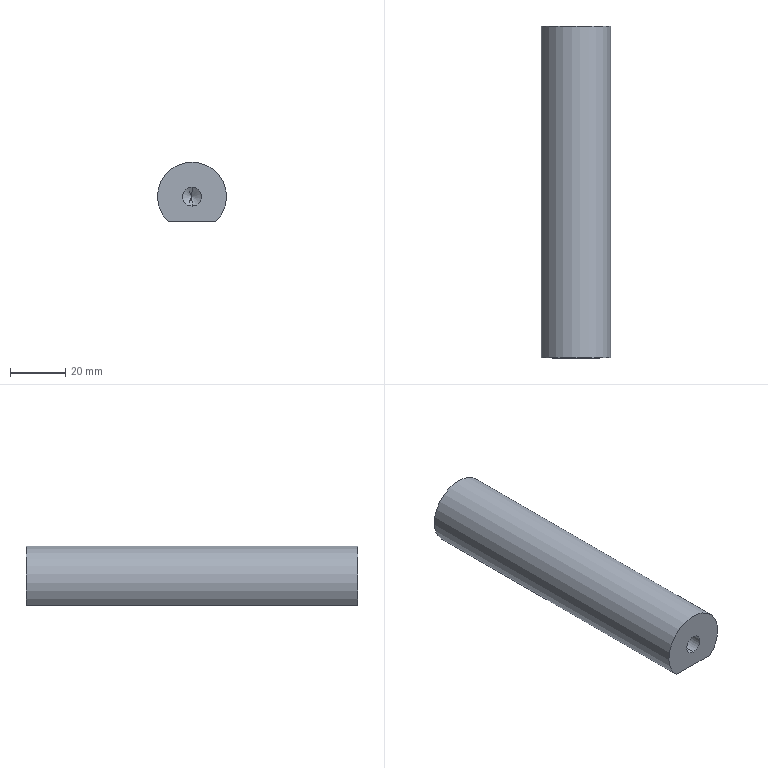Part | STEP file | PN_0003 | 1 solid | 12 faces | box 25 x 120 x 21.5 mm | volume 52408 mm3 | cylinder 5 | cone 4 | plane 3 | commonest cylinder face diameters 6.8 x4 25 x1
STEP:
#1=CARTESIAN_POINT('',(0.,0.,0.));
#2=DIRECTION('',(0.,0.,1.));
#3=DIRECTION('',(1.,0.,0.));
#4=AXIS2_PLACEMENT_3D('',#1,#2,#3);
#5=CARTESIAN_POINT('',(0.,19.75,-3.4));
#6=VERTEX_POINT('',#5);
#7=CARTESIAN_POINT('',(0.,0.,-3.4));
#8=VERTEX_POINT('',#7);
#9=CARTESIAN_POINT('',(0.,0.,-3.4));
#10=DIRECTION('',(0.,-1.,0.));
#11=VECTOR('',#10,1.);
#12=LINE('',#9,#11);
#13=CARTESIAN_POINT('',(0.,0.,0.));
#14=DIRECTION('',(0.,-1.,0.));
#15=DIRECTION('',(0.,0.,-1.));
#16=AXIS2_PLACEMENT_3D('',#13,#14,#15);
#17=CYLINDRICAL_SURFACE('',#16,3.4);
#18=CARTESIAN_POINT('',(6.283,0.));
#19=DIRECTION('',(0.,1.));
#20=VECTOR('',#19,1.);
#21=LINE('',#18,#20);
#22=(GEOMETRIC_REPRESENTATION_CONTEXT(2)PARAMETRIC_REPRESENTATION_CONTEXT()REPRESENTATION_CONTEXT('',''));
#23=DEFINITIONAL_REPRESENTATION('',(#21),#22);
#24=PCURVE('',#17,#23);
#25=CARTESIAN_POINT('',(0.,0.,0.));
#26=DIRECTION('',(0.,-1.,0.));
#27=DIRECTION('',(0.,0.,-1.));
#28=AXIS2_PLACEMENT_3D('',#25,#26,#27);
#29=CYLINDRICAL_SURFACE('',#28,3.4);
#30=CARTESIAN_POINT('',(0.,0.));
#31=DIRECTION('',(0.,1.));
#32=VECTOR('',#31,1.);
#33=LINE('',#30,#32);
#34=(GEOMETRIC_REPRESENTATION_CONTEXT(2)PARAMETRIC_REPRESENTATION_CONTEXT()REPRESENTATION_CONTEXT('',''));
#35=DEFINITIONAL_REPRESENTATION('',(#33),#34);
#36=PCURVE('',#29,#35);
#37=SURFACE_CURVE('',#12,(#24,#36),.PCURVE_S1.);
#38=EDGE_CURVE('',#6,#8,#37,.T.);
#39=ORIENTED_EDGE('',*,*,#38,.T.);
#40=CARTESIAN_POINT('',(0.,0.,3.4));
#41=VERTEX_POINT('',#40);
#42=CARTESIAN_POINT('',(0.,0.,0.));
#43=DIRECTION('',(0.,-1.,0.));
#44=DIRECTION('',(0.,0.,-1.));
#45=AXIS2_PLACEMENT_3D('',#42,#43,#44);
#46=CIRCLE('',#45,3.4);
#47=CARTESIAN_POINT('',(0.,0.));
#48=DIRECTION('',(1.,0.));
#49=VECTOR('',#48,1.);
#50=LINE('',#47,#49);
#51=(GEOMETRIC_REPRESENTATION_CONTEXT(2)PARAMETRIC_REPRESENTATION_CONTEXT()REPRESENTATION_CONTEXT('',''));
#52=DEFINITIONAL_REPRESENTATION('',(#50),#51);
#53=PCURVE('',#17,#52);
#54=CARTESIAN_POINT('',(0.,0.,0.));
#55=DIRECTION('',(0.,1.,0.));
#56=DIRECTION('',(0.,0.,1.));
#57=AXIS2_PLACEMENT_3D('',#54,#55,#56);
#58=PLANE('',#57);
#59=CARTESIAN_POINT('',(-3.4,0.));
#60=CARTESIAN_POINT('',(-3.4,5.889));
#61=CARTESIAN_POINT('',(1.7,2.944));
#62=CARTESIAN_POINT('',(6.8,0.));
#63=CARTESIAN_POINT('',(1.7,-2.944));
#64=CARTESIAN_POINT('',(-3.4,-5.889));
#65=CARTESIAN_POINT('',(-3.4,0.));
#66=(BOUNDED_CURVE()B_SPLINE_CURVE(2,(#59,#60,#61,#62,#63,#64,#65),.UNSPECIFIED.,.T.,.F.)B_SPLINE_CURVE_WITH_KNOTS((1,2,2,2,2,1),(-2.094,0.,2.094,4.189,6.283,8.378),.UNSPECIFIED.)CURVE()GEOMETRIC_REPRESENTATION_ITEM()RATIONAL_B_SPLINE_CURVE((1.,0.5,1.,0.5,1.,0.5,1.))REPRESENTATION_ITEM(''));
#67=(GEOMETRIC_REPRESENTATION_CONTEXT(2)PARAMETRIC_REPRESENTATION_CONTEXT()REPRESENTATION_CONTEXT('',''));
#68=DEFINITIONAL_REPRESENTATION('',(#66),#67);
#69=PCURVE('',#58,#68);
#70=SURFACE_CURVE('',#46,(#53,#69),.PCURVE_S1.);
#71=EDGE_CURVE('',#41,#8,#70,.T.);
#72=ORIENTED_EDGE('',*,*,#71,.F.);
#73=CARTESIAN_POINT('',(0.,19.75,3.4));
#74=VERTEX_POINT('',#73);
#75=CARTESIAN_POINT('',(0.,0.,3.4));
#76=DIRECTION('',(0.,-1.,0.));
#77=VECTOR('',#76,1.);
#78=LINE('',#75,#77);
#79=CARTESIAN_POINT('',(3.142,0.));
#80=DIRECTION('',(0.,1.));
#81=VECTOR('',#80,1.);
#82=LINE('',#79,#81);
#83=(GEOMETRIC_REPRESENTATION_CONTEXT(2)PARAMETRIC_REPRESENTATION_CONTEXT()REPRESENTATION_CONTEXT('',''));
#84=DEFINITIONAL_REPRESENTATION('',(#82),#83);
#85=PCURVE('',#17,#84);
#86=CARTESIAN_POINT('',(3.142,0.));
#87=DIRECTION('',(0.,1.));
#88=VECTOR('',#87,1.);
#89=LINE('',#86,#88);
#90=(GEOMETRIC_REPRESENTATION_CONTEXT(2)PARAMETRIC_REPRESENTATION_CONTEXT()REPRESENTATION_CONTEXT('',''));
#91=DEFINITIONAL_REPRESENTATION('',(#89),#90);
#92=PCURVE('',#29,#91);
#93=SURFACE_CURVE('',#78,(#85,#92),.PCURVE_S1.);
#94=EDGE_CURVE('',#74,#41,#93,.T.);
#95=ORIENTED_EDGE('',*,*,#94,.F.);
#96=CARTESIAN_POINT('',(0.,19.75,0.));
#97=DIRECTION('',(0.,-1.,0.));
#98=DIRECTION('',(0.,0.,-1.));
#99=AXIS2_PLACEMENT_3D('',#96,#97,#98);
#100=CIRCLE('',#99,3.4);
#101=CARTESIAN_POINT('',(0.,-19.75));
#102=DIRECTION('',(1.,0.));
#103=VECTOR('',#102,1.);
#104=LINE('',#101,#103);
#105=(GEOMETRIC_REPRESENTATION_CONTEXT(2)PARAMETRIC_REPRESENTATION_CONTEXT()REPRESENTATION_CONTEXT('',''));
#106=DEFINITIONAL_REPRESENTATION('',(#104),#105);
#107=PCURVE('',#17,#106);
#108=CARTESIAN_POINT('',(0.,19.75,0.));
#109=DIRECTION('',(0.,-1.,0.));
#110=DIRECTION('',(0.,0.,-1.));
#111=AXIS2_PLACEMENT_3D('',#108,#109,#110);
#112=CONICAL_SURFACE('',#111,3.4,1.03);
#113=CARTESIAN_POINT('',(0.,0.));
#114=DIRECTION('',(1.,0.));
#115=VECTOR('',#114,1.);
#116=LINE('',#113,#115);
#117=(GEOMETRIC_REPRESENTATION_CONTEXT(2)PARAMETRIC_REPRESENTATION_CONTEXT()REPRESENTATION_CONTEXT('',''));
#118=DEFINITIONAL_REPRESENTATION('',(#116),#117);
#119=PCURVE('',#112,#118);
#120=SURFACE_CURVE('',#100,(#107,#119),.PCURVE_S1.);
#121=EDGE_CURVE('',#74,#6,#120,.T.);
#122=ORIENTED_EDGE('',*,*,#121,.T.);
#123=EDGE_LOOP('',(#39,#72,#95,#122));
#124=FACE_BOUND('',#123,.F.);
#125=ADVANCED_FACE('',(#124),#17,.F.);
#126=ORIENTED_EDGE('',*,*,#121,.F.);
#127=CARTESIAN_POINT('',(0.,21.793,0.));
#128=VERTEX_POINT('',#127);
#129=CARTESIAN_POINT('',(0.,19.75,3.4));
#130=DIRECTION('',(0.,-0.515,0.8572));
#131=VECTOR('',#130,1.);
#132=LINE('',#129,#131);
#133=CARTESIAN_POINT('',(3.142,0.));
#134=DIRECTION('',(0.,1.));
#135=VECTOR('',#134,1.);
#136=LINE('',#133,#135);
#137=(GEOMETRIC_REPRESENTATION_CONTEXT(2)PARAMETRIC_REPRESENTATION_CONTEXT()REPRESENTATION_CONTEXT('',''));
#138=DEFINITIONAL_REPRESENTATION('',(#136),#137);
#139=PCURVE('',#112,#138);
#140=CARTESIAN_POINT('',(0.,19.75,0.));
#141=DIRECTION('',(0.,-1.,0.));
#142=DIRECTION('',(0.,0.,-1.));
#143=AXIS2_PLACEMENT_3D('',#140,#141,#142);
#144=CONICAL_SURFACE('',#143,3.4,1.03);
#145=CARTESIAN_POINT('',(3.142,0.));
#146=DIRECTION('',(0.,1.));
#147=VECTOR('',#146,1.);
#148=LINE('',#145,#147);
#149=(GEOMETRIC_REPRESENTATION_CONTEXT(2)PARAMETRIC_REPRESENTATION_CONTEXT()REPRESENTATION_CONTEXT('',''));
#150=DEFINITIONAL_REPRESENTATION('',(#148),#149);
#151=PCURVE('',#144,#150);
#152=SURFACE_CURVE('',#132,(#139,#151),.PCURVE_S1.);
#153=EDGE_CURVE('',#128,#74,#152,.T.);
#154=ORIENTED_EDGE('',*,*,#153,.F.);
#155=CARTESIAN_POINT('',(0.,19.75,-3.4));
#156=DIRECTION('',(0.,-0.515,-0.8572));
#157=VECTOR('',#156,1.);
#158=LINE('',#155,#157);
#159=CARTESIAN_POINT('',(6.283,0.));
#160=DIRECTION('',(0.,1.));
#161=VECTOR('',#160,1.);
#162=LINE('',#159,#161);
#163=(GEOMETRIC_REPRESENTATION_CONTEXT(2)PARAMETRIC_REPRESENTATION_CONTEXT()REPRESENTATION_CONTEXT('',''));
#164=DEFINITIONAL_REPRESENTATION('',(#162),#163);
#165=PCURVE('',#112,#164);
#166=CARTESIAN_POINT('',(0.,0.));
#167=DIRECTION('',(0.,1.));
#168=VECTOR('',#167,1.);
#169=LINE('',#166,#168);
#170=(GEOMETRIC_REPRESENTATION_CONTEXT(2)PARAMETRIC_REPRESENTATION_CONTEXT()REPRESENTATION_CONTEXT('',''));
#171=DEFINITIONAL_REPRESENTATION('',(#169),#170);
#172=PCURVE('',#144,#171);
#173=SURFACE_CURVE('',#158,(#165,#172),.PCURVE_S1.);
#174=EDGE_CURVE('',#128,#6,#173,.T.);
#175=ORIENTED_EDGE('',*,*,#174,.T.);
#176=EDGE_LOOP('',(#126,#154,#175));
#177=FACE_BOUND('',#176,.F.);
#178=ADVANCED_FACE('',(#177),#112,.F.);
#179=CARTESIAN_POINT('',(0.,100.25,3.398));
#180=VERTEX_POINT('',#179);
#181=CARTESIAN_POINT('',(0.,120.,3.398));
#182=VERTEX_POINT('',#181);
#183=CARTESIAN_POINT('',(0.,120.,3.398));
#184=DIRECTION('',(0.,1.,0.));
#185=VECTOR('',#184,1.);
#186=LINE('',#183,#185);
#187=CARTESIAN_POINT('',(0.,120.,-0.002145));
#188=DIRECTION('',(0.,1.,0.));
#189=DIRECTION('',(0.,0.,1.));
#190=AXIS2_PLACEMENT_3D('',#187,#188,#189);
#191=CYLINDRICAL_SURFACE('',#190,3.4);
#192=CARTESIAN_POINT('',(6.283,0.));
#193=DIRECTION('',(0.,1.));
#194=VECTOR('',#193,1.);
#195=LINE('',#192,#194);
#196=(GEOMETRIC_REPRESENTATION_CONTEXT(2)PARAMETRIC_REPRESENTATION_CONTEXT()REPRESENTATION_CONTEXT('',''));
#197=DEFINITIONAL_REPRESENTATION('',(#195),#196);
#198=PCURVE('',#191,#197);
#199=CARTESIAN_POINT('',(0.,120.,-0.002145));
#200=DIRECTION('',(0.,1.,0.));
#201=DIRECTION('',(0.,0.,1.));
#202=AXIS2_PLACEMENT_3D('',#199,#200,#201);
#203=CYLINDRICAL_SURFACE('',#202,3.4);
#204=CARTESIAN_POINT('',(0.,0.));
#205=DIRECTION('',(0.,1.));
#206=VECTOR('',#205,1.);
#207=LINE('',#204,#206);
#208=(GEOMETRIC_REPRESENTATION_CONTEXT(2)PARAMETRIC_REPRESENTATION_CONTEXT()REPRESENTATION_CONTEXT('',''));
#209=DEFINITIONAL_REPRESENTATION('',(#207),#208);
#210=PCURVE('',#203,#209);
#211=SURFACE_CURVE('',#186,(#198,#210),.PCURVE_S1.);
#212=EDGE_CURVE('',#180,#182,#211,.T.);
#213=ORIENTED_EDGE('',*,*,#212,.T.);
#214=CARTESIAN_POINT('',(0.,120.,-3.402));
#215=VERTEX_POINT('',#214);
#216=CARTESIAN_POINT('',(0.,120.,-0.002145));
#217=DIRECTION('',(0.,1.,0.));
#218=DIRECTION('',(0.,0.,1.));
#219=AXIS2_PLACEMENT_3D('',#216,#217,#218);
#220=CIRCLE('',#219,3.4);
#221=CARTESIAN_POINT('',(0.,0.));
#222=DIRECTION('',(1.,0.));
#223=VECTOR('',#222,1.);
#224=LINE('',#221,#223);
#225=(GEOMETRIC_REPRESENTATION_CONTEXT(2)PARAMETRIC_REPRESENTATION_CONTEXT()REPRESENTATION_CONTEXT('',''));
#226=DEFINITIONAL_REPRESENTATION('',(#224),#225);
#227=PCURVE('',#191,#226);
#228=CARTESIAN_POINT('',(0.,120.,0.));
#229=DIRECTION('',(0.,1.,0.));
#230=DIRECTION('',(0.,0.,1.));
#231=AXIS2_PLACEMENT_3D('',#228,#229,#230);
#232=PLANE('',#231);
#233=CARTESIAN_POINT('',(-0.002145,0.));
#234=DIRECTION('',(1.,0.));
#235=AXIS2_PLACEMENT_2D('',#233,#234);
#236=CIRCLE('',#235,3.4);
#237=(GEOMETRIC_REPRESENTATION_CONTEXT(2)PARAMETRIC_REPRESENTATION_CONTEXT()REPRESENTATION_CONTEXT('',''));
#238=DEFINITIONAL_REPRESENTATION('',(#236),#237);
#239=PCURVE('',#232,#238);
#240=SURFACE_CURVE('',#220,(#227,#239),.PCURVE_S1.);
#241=EDGE_CURVE('',#215,#182,#240,.T.);
#242=ORIENTED_EDGE('',*,*,#241,.F.);
#243=CARTESIAN_POINT('',(0.,100.25,-3.402));
#244=VERTEX_POINT('',#243);
#245=CARTESIAN_POINT('',(0.,120.,-3.402));
#246=DIRECTION('',(0.,1.,0.));
#247=VECTOR('',#246,1.);
#248=LINE('',#245,#247);
#249=CARTESIAN_POINT('',(3.142,0.));
#250=DIRECTION('',(0.,1.));
#251=VECTOR('',#250,1.);
#252=LINE('',#249,#251);
#253=(GEOMETRIC_REPRESENTATION_CONTEXT(2)PARAMETRIC_REPRESENTATION_CONTEXT()REPRESENTATION_CONTEXT('',''));
#254=DEFINITIONAL_REPRESENTATION('',(#252),#253);
#255=PCURVE('',#191,#254);
#256=CARTESIAN_POINT('',(3.142,0.));
#257=DIRECTION('',(0.,1.));
#258=VECTOR('',#257,1.);
#259=LINE('',#256,#258);
#260=(GEOMETRIC_REPRESENTATION_CONTEXT(2)PARAMETRIC_REPRESENTATION_CONTEXT()REPRESENTATION_CONTEXT('',''));
#261=DEFINITIONAL_REPRESENTATION('',(#259),#260);
#262=PCURVE('',#203,#261);
#263=SURFACE_CURVE('',#248,(#255,#262),.PCURVE_S1.);
#264=EDGE_CURVE('',#244,#215,#263,.T.);
#265=ORIENTED_EDGE('',*,*,#264,.F.);
#266=CARTESIAN_POINT('',(0.,100.25,-0.002145));
#267=DIRECTION('',(0.,1.,0.));
#268=DIRECTION('',(0.,0.,1.));
#269=AXIS2_PLACEMENT_3D('',#266,#267,#268);
#270=CIRCLE('',#269,3.4);
#271=CARTESIAN_POINT('',(0.,-19.75));
#272=DIRECTION('',(1.,0.));
#273=VECTOR('',#272,1.);
#274=LINE('',#271,#273);
#275=(GEOMETRIC_REPRESENTATION_CONTEXT(2)PARAMETRIC_REPRESENTATION_CONTEXT()REPRESENTATION_CONTEXT('',''));
#276=DEFINITIONAL_REPRESENTATION('',(#274),#275);
#277=PCURVE('',#191,#276);
#278=CARTESIAN_POINT('',(0.,100.25,-0.002145));
#279=DIRECTION('',(0.,1.,0.));
#280=DIRECTION('',(0.,0.,1.));
#281=AXIS2_PLACEMENT_3D('',#278,#279,#280);
#282=CONICAL_SURFACE('',#281,3.4,1.03);
#283=CARTESIAN_POINT('',(0.,0.));
#284=DIRECTION('',(1.,0.));
#285=VECTOR('',#284,1.);
#286=LINE('',#283,#285);
#287=(GEOMETRIC_REPRESENTATION_CONTEXT(2)PARAMETRIC_REPRESENTATION_CONTEXT()REPRESENTATION_CONTEXT('',''));
#288=DEFINITIONAL_REPRESENTATION('',(#286),#287);
#289=PCURVE('',#282,#288);
#290=SURFACE_CURVE('',#270,(#277,#289),.PCURVE_S1.);
#291=EDGE_CURVE('',#244,#180,#290,.T.);
#292=ORIENTED_EDGE('',*,*,#291,.T.);
#293=EDGE_LOOP('',(#213,#242,#265,#292));
#294=FACE_BOUND('',#293,.F.);
#295=ADVANCED_FACE('',(#294),#191,.F.);
#296=ORIENTED_EDGE('',*,*,#291,.F.);
#297=CARTESIAN_POINT('',(0.,98.207,-0.002145));
#298=VERTEX_POINT('',#297);
#299=CARTESIAN_POINT('',(0.,100.25,-3.402));
#300=DIRECTION('',(0.,0.515,-0.8572));
#301=VECTOR('',#300,1.);
#302=LINE('',#299,#301);
#303=CARTESIAN_POINT('',(3.142,-2.043));
#304=CARTESIAN_POINT('',(3.142,-2.012));
#305=CARTESIAN_POINT('',(3.142,-1.95));
#306=CARTESIAN_POINT('',(3.142,-1.857));
#307=CARTESIAN_POINT('',(3.142,-1.764));
#308=CARTESIAN_POINT('',(3.142,-1.671));
#309=CARTESIAN_POINT('',(3.142,-1.579));
#310=CARTESIAN_POINT('',(3.142,-1.486));
#311=CARTESIAN_POINT('',(3.142,-1.393));
#312=CARTESIAN_POINT('',(3.142,-1.3));
#313=CARTESIAN_POINT('',(3.142,-1.207));
#314=CARTESIAN_POINT('',(3.142,-1.114));
#315=CARTESIAN_POINT('',(3.142,-1.021));
#316=CARTESIAN_POINT('',(3.142,-0.9286));
#317=CARTESIAN_POINT('',(3.142,-0.8357));
#318=CARTESIAN_POINT('',(3.142,-0.7429));
#319=CARTESIAN_POINT('',(3.142,-0.65));
#320=CARTESIAN_POINT('',(3.142,-0.5572));
#321=CARTESIAN_POINT('',(3.142,-0.4643));
#322=CARTESIAN_POINT('',(3.142,-0.3714));
#323=CARTESIAN_POINT('',(3.142,-0.2786));
#324=CARTESIAN_POINT('',(3.142,-0.1857));
#325=CARTESIAN_POINT('',(3.142,-0.09286));
#326=CARTESIAN_POINT('',(3.142,-0.03095));
#327=CARTESIAN_POINT('',(3.142,0.));
#328=B_SPLINE_CURVE_WITH_KNOTS('',3,(#303,#304,#305,#306,#307,#308,#309,#310,#311,#312,#313,#314,#315,#316,#317,#318,#319,#320,#321,#322,#323,#324,#325,#326,#327),.UNSPECIFIED.,.F.,.F.,(4,1,1,1,1,1,1,1,1,1,1,1,1,1,1,1,1,1,1,1,1,1,4),(-3.967,-3.786,-3.606,-3.426,-3.245,-3.065,-2.885,-2.704,-2.524,-2.344,-2.164,-1.983,-1.803,-1.623,-1.442,-1.262,-1.082,-0.9015,-0.7212,-0.5409,-0.3606,-0.1803,0.),.UNSPECIFIED.);
#329=(GEOMETRIC_REPRESENTATION_CONTEXT(2)PARAMETRIC_REPRESENTATION_CONTEXT()REPRESENTATION_CONTEXT('',''));
#330=DEFINITIONAL_REPRESENTATION('',(#328),#329);
#331=PCURVE('',#282,#330);
#332=CARTESIAN_POINT('',(0.,100.25,-0.002145));
#333=DIRECTION('',(0.,1.,0.));
#334=DIRECTION('',(0.,0.,1.));
#335=AXIS2_PLACEMENT_3D('',#332,#333,#334);
#336=CONICAL_SURFACE('',#335,3.4,1.03);
#337=CARTESIAN_POINT('',(3.142,-2.043));
#338=CARTESIAN_POINT('',(3.142,-2.012));
#339=CARTESIAN_POINT('',(3.142,-1.95));
#340=CARTESIAN_POINT('',(3.142,-1.857));
#341=CARTESIAN_POINT('',(3.142,-1.764));
#342=CARTESIAN_POINT('',(3.142,-1.671));
#343=CARTESIAN_POINT('',(3.142,-1.579));
#344=CARTESIAN_POINT('',(3.142,-1.486));
#345=CARTESIAN_POINT('',(3.142,-1.393));
#346=CARTESIAN_POINT('',(3.142,-1.3));
#347=CARTESIAN_POINT('',(3.142,-1.207));
#348=CARTESIAN_POINT('',(3.142,-1.114));
#349=CARTESIAN_POINT('',(3.142,-1.021));
#350=CARTESIAN_POINT('',(3.142,-0.9286));
#351=CARTESIAN_POINT('',(3.142,-0.8357));
#352=CARTESIAN_POINT('',(3.142,-0.7429));
#353=CARTESIAN_POINT('',(3.142,-0.65));
#354=CARTESIAN_POINT('',(3.142,-0.5572));
#355=CARTESIAN_POINT('',(3.142,-0.4643));
#356=CARTESIAN_POINT('',(3.142,-0.3714));
#357=CARTESIAN_POINT('',(3.142,-0.2786));
#358=CARTESIAN_POINT('',(3.142,-0.1857));
#359=CARTESIAN_POINT('',(3.142,-0.09286));
#360=CARTESIAN_POINT('',(3.142,-0.03095));
#361=CARTESIAN_POINT('',(3.142,0.));
#362=B_SPLINE_CURVE_WITH_KNOTS('',3,(#337,#338,#339,#340,#341,#342,#343,#344,#345,#346,#347,#348,#349,#350,#351,#352,#353,#354,#355,#356,#357,#358,#359,#360,#361),.UNSPECIFIED.,.F.,.F.,(4,1,1,1,1,1,1,1,1,1,1,1,1,1,1,1,1,1,1,1,1,1,4),(-3.967,-3.786,-3.606,-3.426,-3.245,-3.065,-2.885,-2.704,-2.524,-2.344,-2.164,-1.983,-1.803,-1.623,-1.442,-1.262,-1.082,-0.9015,-0.7212,-0.5409,-0.3606,-0.1803,0.),.UNSPECIFIED.);
#363=(GEOMETRIC_REPRESENTATION_CONTEXT(2)PARAMETRIC_REPRESENTATION_CONTEXT()REPRESENTATION_CONTEXT('',''));
#364=DEFINITIONAL_REPRESENTATION('',(#362),#363);
#365=PCURVE('',#336,#364);
#366=SURFACE_CURVE('',#302,(#331,#365),.PCURVE_S1.);
#367=EDGE_CURVE('',#298,#244,#366,.T.);
#368=ORIENTED_EDGE('',*,*,#367,.F.);
#369=CARTESIAN_POINT('',(0.,100.25,3.398));
#370=DIRECTION('',(0.,0.515,0.8572));
#371=VECTOR('',#370,1.);
#372=LINE('',#369,#371);
#373=CARTESIAN_POINT('',(6.283,0.));
#374=DIRECTION('',(0.,1.));
#375=VECTOR('',#374,1.);
#376=LINE('',#373,#375);
#377=(GEOMETRIC_REPRESENTATION_CONTEXT(2)PARAMETRIC_REPRESENTATION_CONTEXT()REPRESENTATION_CONTEXT('',''));
#378=DEFINITIONAL_REPRESENTATION('',(#376),#377);
#379=PCURVE('',#282,#378);
#380=CARTESIAN_POINT('',(0.,0.));
#381=DIRECTION('',(0.,1.));
#382=VECTOR('',#381,1.);
#383=LINE('',#380,#382);
#384=(GEOMETRIC_REPRESENTATION_CONTEXT(2)PARAMETRIC_REPRESENTATION_CONTEXT()REPRESENTATION_CONTEXT('',''));
#385=DEFINITIONAL_REPRESENTATION('',(#383),#384);
#386=PCURVE('',#336,#385);
#387=SURFACE_CURVE('',#372,(#379,#386),.PCURVE_S1.);
#388=EDGE_CURVE('',#298,#180,#387,.T.);
#389=ORIENTED_EDGE('',*,*,#388,.T.);
#390=EDGE_LOOP('',(#296,#368,#389));
#391=FACE_BOUND('',#390,.F.);
#392=ADVANCED_FACE('',(#391),#282,.F.);
#393=CARTESIAN_POINT('',(-8.675,0.,-9.));
#394=VERTEX_POINT('',#393);
#395=CARTESIAN_POINT('',(8.675,0.,-9.));
#396=VERTEX_POINT('',#395);
#397=CARTESIAN_POINT('',(0.,0.,0.));
#398=DIRECTION('',(0.,1.,0.));
#399=DIRECTION('',(0.,0.,1.));
#400=AXIS2_PLACEMENT_3D('',#397,#398,#399);
#401=CIRCLE('',#400,12.5);
#402=CARTESIAN_POINT('',(0.,120.,0.));
#403=DIRECTION('',(0.,-1.,0.));
#404=DIRECTION('',(0.,0.,-1.));
#405=AXIS2_PLACEMENT_3D('',#402,#403,#404);
#406=CYLINDRICAL_SURFACE('',#405,12.5);
#407=CARTESIAN_POINT('',(9.425,120.));
#408=DIRECTION('',(-1.,0.));
#409=VECTOR('',#408,1.);
#410=LINE('',#407,#409);
#411=(GEOMETRIC_REPRESENTATION_CONTEXT(2)PARAMETRIC_REPRESENTATION_CONTEXT()REPRESENTATION_CONTEXT('',''));
#412=DEFINITIONAL_REPRESENTATION('',(#410),#411);
#413=PCURVE('',#406,#412);
#414=CARTESIAN_POINT('',(0.,0.));
#415=DIRECTION('',(1.,0.));
#416=AXIS2_PLACEMENT_2D('',#414,#415);
#417=CIRCLE('',#416,12.5);
#418=(GEOMETRIC_REPRESENTATION_CONTEXT(2)PARAMETRIC_REPRESENTATION_CONTEXT()REPRESENTATION_CONTEXT('',''));
#419=DEFINITIONAL_REPRESENTATION('',(#417),#418);
#420=PCURVE('',#58,#419);
#421=SURFACE_CURVE('',#401,(#413,#420),.PCURVE_S1.);
#422=EDGE_CURVE('',#394,#396,#421,.T.);
#423=ORIENTED_EDGE('',*,*,#422,.T.);
#424=CARTESIAN_POINT('',(8.675,120.,-9.));
#425=VERTEX_POINT('',#424);
#426=CARTESIAN_POINT('',(8.675,120.,-9.));
#427=DIRECTION('',(0.,-1.,0.));
#428=VECTOR('',#427,1.);
#429=LINE('',#426,#428);
#430=CARTESIAN_POINT('',(0.767,0.));
#431=DIRECTION('',(0.,1.));
#432=VECTOR('',#431,1.);
#433=LINE('',#430,#432);
#434=(GEOMETRIC_REPRESENTATION_CONTEXT(2)PARAMETRIC_REPRESENTATION_CONTEXT()REPRESENTATION_CONTEXT('',''));
#435=DEFINITIONAL_REPRESENTATION('',(#433),#434);
#436=PCURVE('',#406,#435);
#437=CARTESIAN_POINT('',(-8.675,120.,-9.));
#438=DIRECTION('',(0.,0.,1.));
#439=DIRECTION('',(1.,0.,0.));
#440=AXIS2_PLACEMENT_3D('',#437,#438,#439);
#441=PLANE('',#440);
#442=CARTESIAN_POINT('',(17.349,0.));
#443=DIRECTION('',(0.,-1.));
#444=VECTOR('',#443,1.);
#445=LINE('',#442,#444);
#446=(GEOMETRIC_REPRESENTATION_CONTEXT(2)PARAMETRIC_REPRESENTATION_CONTEXT()REPRESENTATION_CONTEXT('',''));
#447=DEFINITIONAL_REPRESENTATION('',(#445),#446);
#448=PCURVE('',#441,#447);
#449=SURFACE_CURVE('',#429,(#436,#448),.PCURVE_S1.);
#450=EDGE_CURVE('',#425,#396,#449,.T.);
#451=ORIENTED_EDGE('',*,*,#450,.F.);
#452=CARTESIAN_POINT('',(-8.675,120.,-9.));
#453=VERTEX_POINT('',#452);
#454=CARTESIAN_POINT('',(0.,120.,0.));
#455=DIRECTION('',(0.,1.,0.));
#456=DIRECTION('',(0.,0.,1.));
#457=AXIS2_PLACEMENT_3D('',#454,#455,#456);
#458=CIRCLE('',#457,12.5);
#459=CARTESIAN_POINT('',(9.425,0.));
#460=DIRECTION('',(-1.,0.));
#461=VECTOR('',#460,1.);
#462=LINE('',#459,#461);
#463=(GEOMETRIC_REPRESENTATION_CONTEXT(2)PARAMETRIC_REPRESENTATION_CONTEXT()REPRESENTATION_CONTEXT('',''));
#464=DEFINITIONAL_REPRESENTATION('',(#462),#463);
#465=PCURVE('',#406,#464);
#466=CARTESIAN_POINT('',(0.,0.));
#467=DIRECTION('',(1.,0.));
#468=AXIS2_PLACEMENT_2D('',#466,#467);
#469=CIRCLE('',#468,12.5);
#470=(GEOMETRIC_REPRESENTATION_CONTEXT(2)PARAMETRIC_REPRESENTATION_CONTEXT()REPRESENTATION_CONTEXT('',''));
#471=DEFINITIONAL_REPRESENTATION('',(#469),#470);
#472=PCURVE('',#232,#471);
#473=SURFACE_CURVE('',#458,(#465,#472),.PCURVE_S1.);
#474=EDGE_CURVE('',#453,#425,#473,.T.);
#475=ORIENTED_EDGE('',*,*,#474,.F.);
#476=CARTESIAN_POINT('',(-8.675,120.,-9.));
#477=DIRECTION('',(0.,-1.,0.));
#478=VECTOR('',#477,1.);
#479=LINE('',#476,#478);
#480=CARTESIAN_POINT('',(5.516,0.));
#481=DIRECTION('',(0.,1.));
#482=VECTOR('',#481,1.);
#483=LINE('',#480,#482);
#484=(GEOMETRIC_REPRESENTATION_CONTEXT(2)PARAMETRIC_REPRESENTATION_CONTEXT()REPRESENTATION_CONTEXT('',''));
#485=DEFINITIONAL_REPRESENTATION('',(#483),#484);
#486=PCURVE('',#406,#485);
#487=CARTESIAN_POINT('',(0.,0.));
#488=DIRECTION('',(0.,-1.));
#489=VECTOR('',#488,1.);
#490=LINE('',#487,#489);
#491=(GEOMETRIC_REPRESENTATION_CONTEXT(2)PARAMETRIC_REPRESENTATION_CONTEXT()REPRESENTATION_CONTEXT('',''));
#492=DEFINITIONAL_REPRESENTATION('',(#490),#491);
#493=PCURVE('',#441,#492);
#494=SURFACE_CURVE('',#479,(#486,#493),.PCURVE_S1.);
#495=EDGE_CURVE('',#453,#394,#494,.T.);
#496=ORIENTED_EDGE('',*,*,#495,.T.);
#497=EDGE_LOOP('',(#423,#451,#475,#496));
#498=FACE_BOUND('',#497,.T.);
#499=ADVANCED_FACE('',(#498),#406,.T.);
#500=CARTESIAN_POINT('',(-8.675,0.,-9.));
#501=DIRECTION('',(-1.,0.,0.));
#502=VECTOR('',#501,1.);
#503=LINE('',#500,#502);
#504=CARTESIAN_POINT('',(0.,-120.));
#505=DIRECTION('',(-1.,0.));
#506=VECTOR('',#505,1.);
#507=LINE('',#504,#506);
#508=(GEOMETRIC_REPRESENTATION_CONTEXT(2)PARAMETRIC_REPRESENTATION_CONTEXT()REPRESENTATION_CONTEXT('',''));
#509=DEFINITIONAL_REPRESENTATION('',(#507),#508);
#510=PCURVE('',#441,#509);
#511=CARTESIAN_POINT('',(-9.,-8.675));
#512=DIRECTION('',(0.,-1.));
#513=VECTOR('',#512,1.);
#514=LINE('',#511,#513);
#515=(GEOMETRIC_REPRESENTATION_CONTEXT(2)PARAMETRIC_REPRESENTATION_CONTEXT()REPRESENTATION_CONTEXT('',''));
#516=DEFINITIONAL_REPRESENTATION('',(#514),#515);
#517=PCURVE('',#58,#516);
#518=SURFACE_CURVE('',#503,(#510,#517),.PCURVE_S1.);
#519=EDGE_CURVE('',#396,#394,#518,.T.);
#520=ORIENTED_EDGE('',*,*,#519,.T.);
#521=ORIENTED_EDGE('',*,*,#495,.F.);
#522=CARTESIAN_POINT('',(-8.675,120.,-9.));
#523=DIRECTION('',(-1.,0.,0.));
#524=VECTOR('',#523,1.);
#525=LINE('',#522,#524);
#526=CARTESIAN_POINT('',(0.,0.));
#527=DIRECTION('',(-1.,0.));
#528=VECTOR('',#527,1.);
#529=LINE('',#526,#528);
#530=(GEOMETRIC_REPRESENTATION_CONTEXT(2)PARAMETRIC_REPRESENTATION_CONTEXT()REPRESENTATION_CONTEXT('',''));
#531=DEFINITIONAL_REPRESENTATION('',(#529),#530);
#532=PCURVE('',#441,#531);
#533=CARTESIAN_POINT('',(-9.,-8.675));
#534=DIRECTION('',(0.,-1.));
#535=VECTOR('',#534,1.);
#536=LINE('',#533,#535);
#537=(GEOMETRIC_REPRESENTATION_CONTEXT(2)PARAMETRIC_REPRESENTATION_CONTEXT()REPRESENTATION_CONTEXT('',''));
#538=DEFINITIONAL_REPRESENTATION('',(#536),#537);
#539=PCURVE('',#232,#538);
#540=SURFACE_CURVE('',#525,(#532,#539),.PCURVE_S1.);
#541=EDGE_CURVE('',#425,#453,#540,.T.);
#542=ORIENTED_EDGE('',*,*,#541,.F.);
#543=ORIENTED_EDGE('',*,*,#450,.T.);
#544=EDGE_LOOP('',(#520,#521,#542,#543));
#545=FACE_BOUND('',#544,.T.);
#546=ADVANCED_FACE('',(#545),#441,.F.);
#547=CARTESIAN_POINT('',(0.,120.,-0.002145));
#548=DIRECTION('',(0.,1.,0.));
#549=DIRECTION('',(0.,0.,1.));
#550=AXIS2_PLACEMENT_3D('',#547,#548,#549);
#551=CIRCLE('',#550,3.4);
#552=CARTESIAN_POINT('',(-0.002145,0.));
#553=DIRECTION('',(1.,0.));
#554=AXIS2_PLACEMENT_2D('',#552,#553);
#555=CIRCLE('',#554,3.4);
#556=(GEOMETRIC_REPRESENTATION_CONTEXT(2)PARAMETRIC_REPRESENTATION_CONTEXT()REPRESENTATION_CONTEXT('',''));
#557=DEFINITIONAL_REPRESENTATION('',(#555),#556);
#558=PCURVE('',#232,#557);
#559=CARTESIAN_POINT('',(0.,0.));
#560=DIRECTION('',(1.,0.));
#561=VECTOR('',#560,1.);
#562=LINE('',#559,#561);
#563=(GEOMETRIC_REPRESENTATION_CONTEXT(2)PARAMETRIC_REPRESENTATION_CONTEXT()REPRESENTATION_CONTEXT('',''));
#564=DEFINITIONAL_REPRESENTATION('',(#562),#563);
#565=PCURVE('',#203,#564);
#566=SURFACE_CURVE('',#551,(#558,#565),.PCURVE_S1.);
#567=EDGE_CURVE('',#182,#215,#566,.T.);
#568=ORIENTED_EDGE('',*,*,#567,.F.);
#569=ORIENTED_EDGE('',*,*,#241,.F.);
#570=EDGE_LOOP('',(#568,#569));
#571=FACE_BOUND('',#570,.T.);
#572=ORIENTED_EDGE('',*,*,#474,.T.);
#573=ORIENTED_EDGE('',*,*,#541,.T.);
#574=EDGE_LOOP('',(#572,#573));
#575=FACE_BOUND('',#574,.T.);
#576=ADVANCED_FACE('',(#571,#575),#232,.T.);
#577=CARTESIAN_POINT('',(0.,0.,0.));
#578=DIRECTION('',(0.,-1.,0.));
#579=DIRECTION('',(0.,0.,-1.));
#580=AXIS2_PLACEMENT_3D('',#577,#578,#579);
#581=CIRCLE('',#580,3.4);
#582=CARTESIAN_POINT('',(-3.4,0.));
#583=CARTESIAN_POINT('',(-3.4,5.889));
#584=CARTESIAN_POINT('',(1.7,2.944));
#585=CARTESIAN_POINT('',(6.8,0.));
#586=CARTESIAN_POINT('',(1.7,-2.944));
#587=CARTESIAN_POINT('',(-3.4,-5.889));
#588=CARTESIAN_POINT('',(-3.4,0.));
#589=(BOUNDED_CURVE()B_SPLINE_CURVE(2,(#582,#583,#584,#585,#586,#587,#588),.UNSPECIFIED.,.T.,.F.)B_SPLINE_CURVE_WITH_KNOTS((1,2,2,2,2,1),(-2.094,0.,2.094,4.189,6.283,8.378),.UNSPECIFIED.)CURVE()GEOMETRIC_REPRESENTATION_ITEM()RATIONAL_B_SPLINE_CURVE((1.,0.5,1.,0.5,1.,0.5,1.))REPRESENTATION_ITEM(''));
#590=(GEOMETRIC_REPRESENTATION_CONTEXT(2)PARAMETRIC_REPRESENTATION_CONTEXT()REPRESENTATION_CONTEXT('',''));
#591=DEFINITIONAL_REPRESENTATION('',(#589),#590);
#592=PCURVE('',#58,#591);
#593=CARTESIAN_POINT('',(0.,0.));
#594=DIRECTION('',(1.,0.));
#595=VECTOR('',#594,1.);
#596=LINE('',#593,#595);
#597=(GEOMETRIC_REPRESENTATION_CONTEXT(2)PARAMETRIC_REPRESENTATION_CONTEXT()REPRESENTATION_CONTEXT('',''));
#598=DEFINITIONAL_REPRESENTATION('',(#596),#597);
#599=PCURVE('',#29,#598);
#600=SURFACE_CURVE('',#581,(#592,#599),.PCURVE_S1.);
#601=EDGE_CURVE('',#8,#41,#600,.T.);
#602=ORIENTED_EDGE('',*,*,#601,.F.);
#603=ORIENTED_EDGE('',*,*,#71,.F.);
#604=EDGE_LOOP('',(#602,#603));
#605=FACE_BOUND('',#604,.T.);
#606=ORIENTED_EDGE('',*,*,#422,.F.);
#607=ORIENTED_EDGE('',*,*,#519,.F.);
#608=EDGE_LOOP('',(#606,#607));
#609=FACE_BOUND('',#608,.T.);
#610=ADVANCED_FACE('',(#605,#609),#58,.F.);
#611=CARTESIAN_POINT('',(0.,100.25,-0.002145));
#612=DIRECTION('',(0.,1.,0.));
#613=DIRECTION('',(0.,0.,1.));
#614=AXIS2_PLACEMENT_3D('',#611,#612,#613);
#615=CIRCLE('',#614,3.4);
#616=CARTESIAN_POINT('',(0.,0.));
#617=DIRECTION('',(1.,0.));
#618=VECTOR('',#617,1.);
#619=LINE('',#616,#618);
#620=(GEOMETRIC_REPRESENTATION_CONTEXT(2)PARAMETRIC_REPRESENTATION_CONTEXT()REPRESENTATION_CONTEXT('',''));
#621=DEFINITIONAL_REPRESENTATION('',(#619),#620);
#622=PCURVE('',#336,#621);
#623=CARTESIAN_POINT('',(0.,-19.75));
#624=DIRECTION('',(1.,0.));
#625=VECTOR('',#624,1.);
#626=LINE('',#623,#625);
#627=(GEOMETRIC_REPRESENTATION_CONTEXT(2)PARAMETRIC_REPRESENTATION_CONTEXT()REPRESENTATION_CONTEXT('',''));
#628=DEFINITIONAL_REPRESENTATION('',(#626),#627);
#629=PCURVE('',#203,#628);
#630=SURFACE_CURVE('',#615,(#622,#629),.PCURVE_S1.);
#631=EDGE_CURVE('',#180,#244,#630,.T.);
#632=ORIENTED_EDGE('',*,*,#631,.F.);
#633=ORIENTED_EDGE('',*,*,#388,.F.);
#634=ORIENTED_EDGE('',*,*,#367,.T.);
#635=EDGE_LOOP('',(#632,#633,#634));
#636=FACE_BOUND('',#635,.F.);
#637=ADVANCED_FACE('',(#636),#336,.F.);
#638=ORIENTED_EDGE('',*,*,#567,.F.);
#639=ORIENTED_EDGE('',*,*,#212,.F.);
#640=ORIENTED_EDGE('',*,*,#631,.T.);
#641=ORIENTED_EDGE('',*,*,#264,.T.);
#642=EDGE_LOOP('',(#638,#639,#640,#641));
#643=FACE_BOUND('',#642,.F.);
#644=ADVANCED_FACE('',(#643),#203,.F.);
#645=CARTESIAN_POINT('',(0.,19.75,0.));
#646=DIRECTION('',(0.,-1.,0.));
#647=DIRECTION('',(0.,0.,-1.));
#648=AXIS2_PLACEMENT_3D('',#645,#646,#647);
#649=CIRCLE('',#648,3.4);
#650=CARTESIAN_POINT('',(0.,0.));
#651=DIRECTION('',(1.,0.));
#652=VECTOR('',#651,1.);
#653=LINE('',#650,#652);
#654=(GEOMETRIC_REPRESENTATION_CONTEXT(2)PARAMETRIC_REPRESENTATION_CONTEXT()REPRESENTATION_CONTEXT('',''));
#655=DEFINITIONAL_REPRESENTATION('',(#653),#654);
#656=PCURVE('',#144,#655);
#657=CARTESIAN_POINT('',(0.,-19.75));
#658=DIRECTION('',(1.,0.));
#659=VECTOR('',#658,1.);
#660=LINE('',#657,#659);
#661=(GEOMETRIC_REPRESENTATION_CONTEXT(2)PARAMETRIC_REPRESENTATION_CONTEXT()REPRESENTATION_CONTEXT('',''));
#662=DEFINITIONAL_REPRESENTATION('',(#660),#661);
#663=PCURVE('',#29,#662);
#664=SURFACE_CURVE('',#649,(#656,#663),.PCURVE_S1.);
#665=EDGE_CURVE('',#6,#74,#664,.T.);
#666=ORIENTED_EDGE('',*,*,#665,.F.);
#667=ORIENTED_EDGE('',*,*,#174,.F.);
#668=ORIENTED_EDGE('',*,*,#153,.T.);
#669=EDGE_LOOP('',(#666,#667,#668));
#670=FACE_BOUND('',#669,.F.);
#671=ADVANCED_FACE('',(#670),#144,.F.);
#672=ORIENTED_EDGE('',*,*,#601,.F.);
#673=ORIENTED_EDGE('',*,*,#38,.F.);
#674=ORIENTED_EDGE('',*,*,#665,.T.);
#675=ORIENTED_EDGE('',*,*,#94,.T.);
#676=EDGE_LOOP('',(#672,#673,#674,#675));
#677=FACE_BOUND('',#676,.F.);
#678=ADVANCED_FACE('',(#677),#29,.F.);
#679=CLOSED_SHELL('',(#125,#178,#295,#392,#499,#546,#576,#610,#637,#644,#671,#678));
#680=MANIFOLD_SOLID_BREP('',#679);
#681=(LENGTH_UNIT()NAMED_UNIT(*)SI_UNIT(.MILLI.,.METRE.));
#682=UNCERTAINTY_MEASURE_WITH_UNIT(LENGTH_MEASURE(0.0000001),#681,'','');
#683=(NAMED_UNIT(*)PLANE_ANGLE_UNIT()SI_UNIT($,.RADIAN.));
#684=(NAMED_UNIT(*)SI_UNIT($,.STERADIAN.)SOLID_ANGLE_UNIT());
#685=(GEOMETRIC_REPRESENTATION_CONTEXT(3)GLOBAL_UNCERTAINTY_ASSIGNED_CONTEXT((#682))GLOBAL_UNIT_ASSIGNED_CONTEXT((#681,#683,#684))REPRESENTATION_CONTEXT('',''));
#686=ADVANCED_BREP_SHAPE_REPRESENTATION('',(#4,#680),#685);